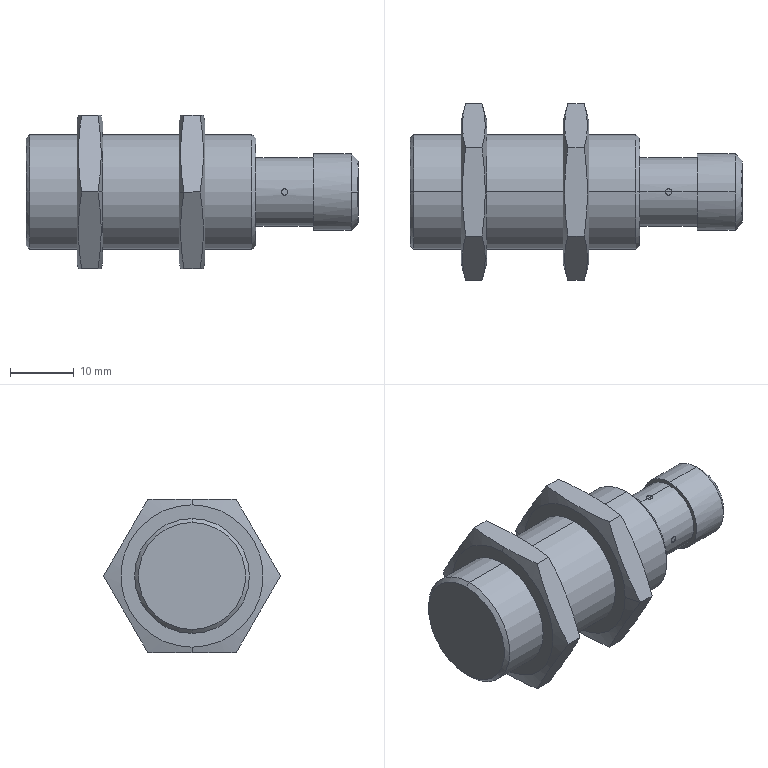Part | STEP file | 4 solids | 81 faces | box 52 x 27.713 x 24 mm | volume 12410 mm3 | cylinder 33 | plane 26 | cone 22 | commonest cylinder face diameters 1 x16 10.6 x5 16.917 x4 9.6 x2 10.8 x2 12 x2